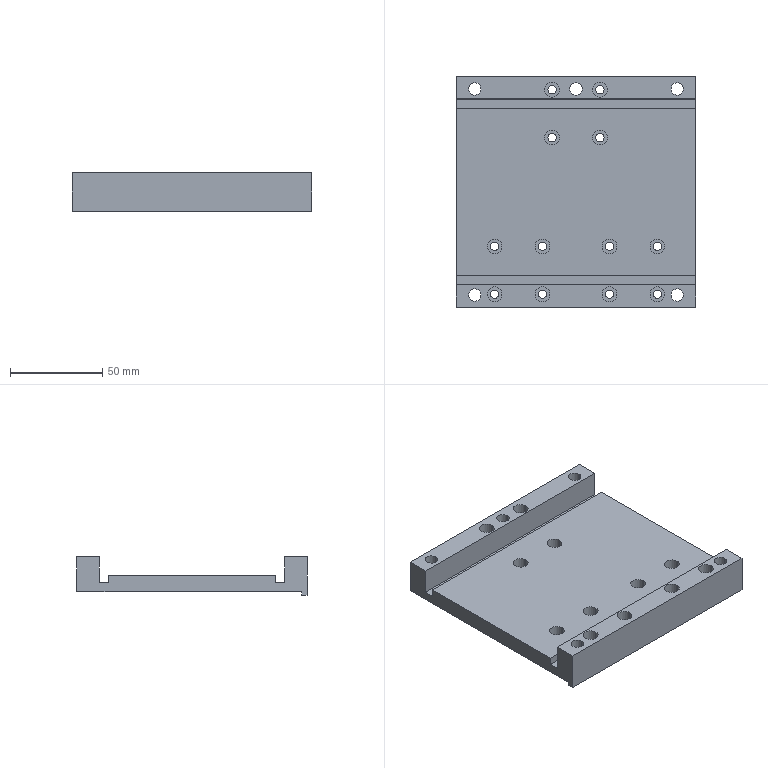Part | STEP file | Crossbeam slider connecting plate | 1 solid | 86 faces | box 130 x 125 x 21 mm | volume 162372 mm3 | cylinder 58 | plane 28 | commonest cylinder face diameters 4.5 x24 8 x24 6.8 x10